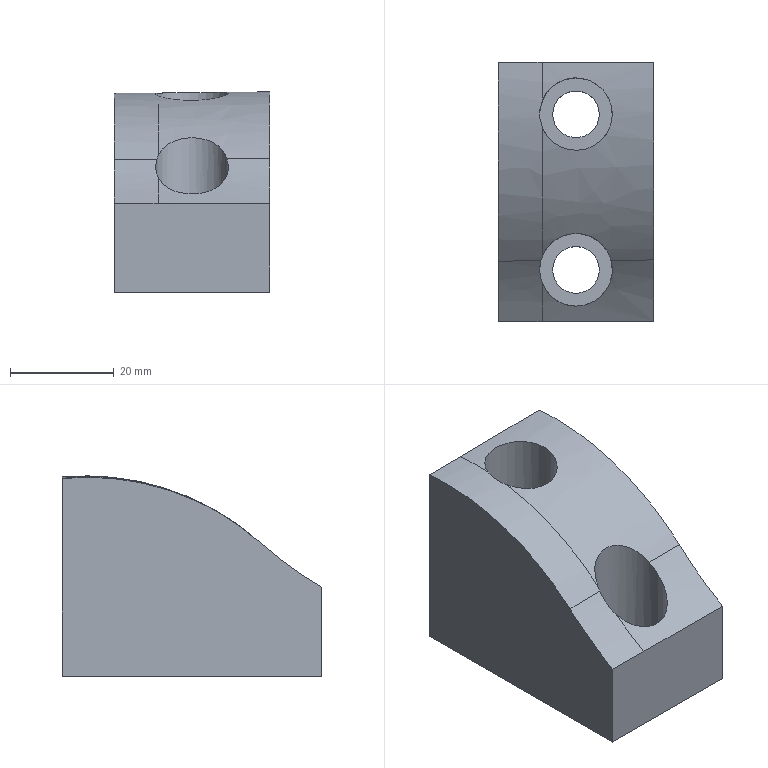Part | NX | features solid 2 | 1 solid | 15 faces | box 30 x 50 x 38.612 mm | volume 39721 mm3 | plane 7 | cylinder 4 | spline 4 | commonest cylinder face diameters 9 x2 14 x2
STEP:
#1=CARTESIAN_POINT('',(470.,654.163,-43.399));
#2=VERTEX_POINT('',#1);
#3=CARTESIAN_POINT('',(470.,642.5,-51.831));
#4=VERTEX_POINT('',#3);
#5=CARTESIAN_POINT('',(470.,654.163,-43.399));
#6=CARTESIAN_POINT('',(470.,650.566,-46.612));
#7=CARTESIAN_POINT('',(470.,646.678,-49.423));
#8=CARTESIAN_POINT('',(470.,642.5,-51.831));
#9=B_SPLINE_CURVE_WITH_KNOTS('',3,(#5,#6,#7,#8),.UNSPECIFIED.,.F.,.F.,(4,4),(0.,0.01439),.UNSPECIFIED.);
#10=EDGE_CURVE('',#2,#4,#9,.T.);
#11=ORIENTED_EDGE('',*,*,#10,.F.);
#12=CARTESIAN_POINT('',(470.,692.5,-30.941));
#13=VERTEX_POINT('',#12);
#14=CARTESIAN_POINT('',(470.,654.163,-43.399));
#15=CARTESIAN_POINT('',(470.,656.729,-41.108));
#16=CARTESIAN_POINT('',(470.,662.388,-37.023));
#17=CARTESIAN_POINT('',(470.,671.861,-32.81));
#18=CARTESIAN_POINT('',(470.,682.125,-30.614));
#19=CARTESIAN_POINT('',(470.,689.029,-30.591));
#20=CARTESIAN_POINT('',(470.,692.5,-30.941));
#21=B_SPLINE_CURVE_WITH_KNOTS('',3,(#14,#15,#16,#17,#18,#19,#20),.UNSPECIFIED.,.F.,.F.,(4,1,1,1,4),(0.007147,0.01746,0.02778,0.0381,0.04842),.UNSPECIFIED.);
#22=EDGE_CURVE('',#2,#13,#21,.T.);
#23=ORIENTED_EDGE('',*,*,#22,.T.);
#24=CARTESIAN_POINT('',(470.,692.5,-69.));
#25=VERTEX_POINT('',#24);
#26=CARTESIAN_POINT('',(470.,692.5,26.));
#27=DIRECTION('',(0.,0.,-1.));
#28=VECTOR('',#27,1000.);
#29=LINE('',#26,#28);
#30=EDGE_CURVE('',#13,#25,#29,.T.);
#31=ORIENTED_EDGE('',*,*,#30,.T.);
#32=CARTESIAN_POINT('',(470.,642.5,-69.));
#33=VERTEX_POINT('',#32);
#34=CARTESIAN_POINT('',(470.,692.5,-69.));
#35=DIRECTION('',(0.,-1.,0.));
#36=VECTOR('',#35,1000.);
#37=LINE('',#34,#36);
#38=EDGE_CURVE('',#25,#33,#37,.T.);
#39=ORIENTED_EDGE('',*,*,#38,.T.);
#40=CARTESIAN_POINT('',(470.,642.5,26.));
#41=DIRECTION('',(0.,0.,-1.));
#42=VECTOR('',#41,1000.);
#43=LINE('',#40,#42);
#44=EDGE_CURVE('',#4,#33,#43,.T.);
#45=ORIENTED_EDGE('',*,*,#44,.F.);
#46=EDGE_LOOP('',(#11,#23,#31,#39,#45));
#47=FACE_BOUND('',#46,.T.);
#48=CARTESIAN_POINT('',(470.,692.5,26.));
#49=DIRECTION('',(1.,0.,0.));
#50=DIRECTION('',(0.,0.,-1.));
#51=AXIS2_PLACEMENT_3D('',#48,#49,#50);
#52=PLANE('',#51);
#53=ADVANCED_FACE('',(#47),#52,.F.);
#54=CARTESIAN_POINT('',(500.,692.5,-30.601));
#55=VERTEX_POINT('',#54);
#56=CARTESIAN_POINT('',(500.,692.5,-69.));
#57=VERTEX_POINT('',#56);
#58=CARTESIAN_POINT('',(500.,692.5,26.));
#59=DIRECTION('',(0.,0.,-1.));
#60=VECTOR('',#59,1000.);
#61=LINE('',#58,#60);
#62=EDGE_CURVE('',#55,#57,#61,.T.);
#63=ORIENTED_EDGE('',*,*,#62,.F.);
#64=CARTESIAN_POINT('',(500.,654.387,-43.29));
#65=VERTEX_POINT('',#64);
#66=CARTESIAN_POINT('',(500.,692.5,-30.601));
#67=CARTESIAN_POINT('',(500.,689.038,-30.282));
#68=CARTESIAN_POINT('',(500.,682.189,-30.36));
#69=CARTESIAN_POINT('',(500.,671.967,-32.624));
#70=CARTESIAN_POINT('',(500.,662.587,-36.865));
#71=CARTESIAN_POINT('',(500.,656.939,-40.985));
#72=CARTESIAN_POINT('',(500.,654.387,-43.291));
#73=B_SPLINE_CURVE_WITH_KNOTS('',3,(#66,#67,#68,#69,#70,#71,#72),.UNSPECIFIED.,.F.,.F.,(4,1,1,1,4),(0.,0.01028,0.02056,0.03084,0.04112),.UNSPECIFIED.);
#74=EDGE_CURVE('',#55,#65,#73,.T.);
#75=ORIENTED_EDGE('',*,*,#74,.T.);
#76=CARTESIAN_POINT('',(500.,642.5,-51.947));
#77=VERTEX_POINT('',#76);
#78=CARTESIAN_POINT('',(500.,642.5,-51.947));
#79=CARTESIAN_POINT('',(500.,646.767,-49.48));
#80=CARTESIAN_POINT('',(500.,650.73,-46.594));
#81=CARTESIAN_POINT('',(500.,654.387,-43.29));
#82=B_SPLINE_CURVE_WITH_KNOTS('',3,(#78,#79,#80,#81),.UNSPECIFIED.,.F.,.F.,(4,4),(0.,0.01471),.UNSPECIFIED.);
#83=EDGE_CURVE('',#77,#65,#82,.T.);
#84=ORIENTED_EDGE('',*,*,#83,.F.);
#85=CARTESIAN_POINT('',(500.,642.5,-69.));
#86=VERTEX_POINT('',#85);
#87=CARTESIAN_POINT('',(500.,642.5,26.));
#88=DIRECTION('',(0.,0.,-1.));
#89=VECTOR('',#88,1000.);
#90=LINE('',#87,#89);
#91=EDGE_CURVE('',#77,#86,#90,.T.);
#92=ORIENTED_EDGE('',*,*,#91,.T.);
#93=CARTESIAN_POINT('',(500.,692.5,-69.));
#94=DIRECTION('',(0.,1.,0.));
#95=VECTOR('',#94,1000.);
#96=LINE('',#93,#95);
#97=EDGE_CURVE('',#57,#86,#96,.F.);
#98=ORIENTED_EDGE('',*,*,#97,.F.);
#99=EDGE_LOOP('',(#63,#75,#84,#92,#98));
#100=FACE_BOUND('',#99,.T.);
#101=CARTESIAN_POINT('',(500.,692.5,26.));
#102=DIRECTION('',(1.,0.,0.));
#103=DIRECTION('',(0.,0.,-1.));
#104=AXIS2_PLACEMENT_3D('',#101,#102,#103);
#105=PLANE('',#104);
#106=ADVANCED_FACE('',(#100),#105,.T.);
#107=CARTESIAN_POINT('',(478.461,692.5,-30.845));
#108=VERTEX_POINT('',#107);
#109=CARTESIAN_POINT('',(470.,692.5,-30.941));
#110=CARTESIAN_POINT('',(472.82,692.5,-30.909));
#111=CARTESIAN_POINT('',(475.641,692.5,-30.877));
#112=CARTESIAN_POINT('',(478.461,692.5,-30.845));
#113=B_SPLINE_CURVE_WITH_KNOTS('',3,(#109,#110,#111,#112),.UNSPECIFIED.,.F.,.F.,(4,4),(0.,0.008461),.UNSPECIFIED.);
#114=EDGE_CURVE('',#13,#108,#113,.T.);
#115=ORIENTED_EDGE('',*,*,#114,.T.);
#116=CARTESIAN_POINT('',(478.461,692.5,-30.845));
#117=CARTESIAN_POINT('',(485.641,692.5,-30.764));
#118=CARTESIAN_POINT('',(492.82,692.5,-30.683));
#119=CARTESIAN_POINT('',(500.,692.5,-30.601));
#120=B_SPLINE_CURVE_WITH_KNOTS('',3,(#116,#117,#118,#119),.UNSPECIFIED.,.F.,.F.,(4,4),(0.001781,0.02332),.UNSPECIFIED.);
#121=EDGE_CURVE('',#108,#55,#120,.T.);
#122=ORIENTED_EDGE('',*,*,#121,.T.);
#123=ORIENTED_EDGE('',*,*,#62,.T.);
#124=CARTESIAN_POINT('',(470.,692.5,-69.));
#125=DIRECTION('',(-1.,0.,0.));
#126=VECTOR('',#125,1000.);
#127=LINE('',#124,#126);
#128=EDGE_CURVE('',#25,#57,#127,.F.);
#129=ORIENTED_EDGE('',*,*,#128,.F.);
#130=ORIENTED_EDGE('',*,*,#30,.F.);
#131=EDGE_LOOP('',(#115,#122,#123,#129,#130));
#132=FACE_BOUND('',#131,.T.);
#133=CARTESIAN_POINT('',(470.,692.5,26.));
#134=DIRECTION('',(0.,1.,0.));
#135=DIRECTION('',(0.,0.,-1.));
#136=AXIS2_PLACEMENT_3D('',#133,#134,#135);
#137=PLANE('',#136);
#138=ADVANCED_FACE('',(#132),#137,.T.);
#139=CARTESIAN_POINT('',(478.,682.5,-59.));
#140=VERTEX_POINT('',#139);
#141=CARTESIAN_POINT('',(485.,682.5,-59.));
#142=DIRECTION('',(0.,0.,-1.));
#143=DIRECTION('',(-1.,0.,0.));
#144=AXIS2_PLACEMENT_3D('',#141,#142,#143);
#145=CIRCLE('',#144,7.);
#146=EDGE_CURVE('',#140,#140,#145,.T.);
#147=ORIENTED_EDGE('',*,*,#146,.T.);
#148=EDGE_LOOP('',(#147));
#149=FACE_BOUND('',#148,.T.);
#150=CARTESIAN_POINT('',(478.461,684.998,-30.673));
#151=VERTEX_POINT('',#150);
#152=CARTESIAN_POINT('',(478.461,680.002,-31.186));
#153=VERTEX_POINT('',#152);
#154=CARTESIAN_POINT('',(478.461,684.998,-30.673));
#155=CARTESIAN_POINT('',(479.04,686.514,-30.589));
#156=CARTESIAN_POINT('',(481.299,689.126,-30.582));
#157=CARTESIAN_POINT('',(486.414,689.957,-30.579));
#158=CARTESIAN_POINT('',(490.872,687.312,-30.43));
#159=CARTESIAN_POINT('',(492.581,682.42,-30.663));
#160=CARTESIAN_POINT('',(490.801,677.632,-31.471));
#161=CARTESIAN_POINT('',(486.374,675.036,-32.165));
#162=CARTESIAN_POINT('',(481.246,675.906,-31.954));
#163=CARTESIAN_POINT('',(479.033,678.504,-31.412));
#164=CARTESIAN_POINT('',(478.461,680.002,-31.186));
#165=B_SPLINE_CURVE_WITH_KNOTS('',3,(#154,#155,#156,#157,#158,#159,#160,#161,#162,#163,#164),.UNSPECIFIED.,.F.,.F.,(4,1,1,1,1,1,1,1,4),(0.01357,0.01842,0.02328,0.02813,0.03298,0.03784,0.04269,0.04755,0.0524),.UNSPECIFIED.);
#166=EDGE_CURVE('',#151,#153,#165,.T.);
#167=ORIENTED_EDGE('',*,*,#166,.F.);
#168=CARTESIAN_POINT('',(478.461,680.002,-31.186));
#169=CARTESIAN_POINT('',(477.855,681.588,-30.947));
#170=CARTESIAN_POINT('',(477.852,683.405,-30.762));
#171=CARTESIAN_POINT('',(478.461,684.998,-30.673));
#172=B_SPLINE_CURVE_WITH_KNOTS('',3,(#168,#169,#170,#171),.UNSPECIFIED.,.F.,.F.,(4,4),(0.0028,0.007913),.UNSPECIFIED.);
#173=EDGE_CURVE('',#153,#151,#172,.T.);
#174=ORIENTED_EDGE('',*,*,#173,.F.);
#175=EDGE_LOOP('',(#167,#174));
#176=FACE_BOUND('',#175,.T.);
#177=CARTESIAN_POINT('',(485.,682.5,26.));
#178=DIRECTION('',(0.,0.,-1.));
#179=DIRECTION('',(0.,-1.,0.));
#180=AXIS2_PLACEMENT_3D('',#177,#178,#179);
#181=CYLINDRICAL_SURFACE('',#180,7.);
#182=ADVANCED_FACE('',(#149,#176),#181,.F.);
#183=CARTESIAN_POINT('',(478.,652.5,-59.));
#184=VERTEX_POINT('',#183);
#185=CARTESIAN_POINT('',(485.,652.5,-59.));
#186=DIRECTION('',(0.,0.,-1.));
#187=DIRECTION('',(-1.,0.,0.));
#188=AXIS2_PLACEMENT_3D('',#185,#186,#187);
#189=CIRCLE('',#188,7.);
#190=EDGE_CURVE('',#184,#184,#189,.T.);
#191=ORIENTED_EDGE('',*,*,#190,.T.);
#192=EDGE_LOOP('',(#191));
#193=FACE_BOUND('',#192,.T.);
#194=CARTESIAN_POINT('',(478.461,654.998,-42.695));
#195=VERTEX_POINT('',#194);
#196=CARTESIAN_POINT('',(491.756,654.33,-43.319));
#197=VERTEX_POINT('',#196);
#198=CARTESIAN_POINT('',(478.461,654.998,-42.695));
#199=CARTESIAN_POINT('',(478.914,656.184,-41.676));
#200=CARTESIAN_POINT('',(480.555,658.558,-39.864));
#201=CARTESIAN_POINT('',(484.662,659.839,-39.021));
#202=CARTESIAN_POINT('',(487.869,659.033,-39.565));
#203=CARTESIAN_POINT('',(490.441,657.323,-40.794));
#204=CARTESIAN_POINT('',(491.434,655.52,-42.247));
#205=CARTESIAN_POINT('',(491.756,654.33,-43.32));
#206=B_SPLINE_CURVE_WITH_KNOTS('',3,(#198,#199,#200,#201,#202,#203,#204,#205),.UNSPECIFIED.,.F.,.F.,(4,1,1,1,1,4),(0.008202,0.01303,0.01785,0.02027,0.02268,0.02751),.UNSPECIFIED.);
#207=EDGE_CURVE('',#195,#197,#206,.T.);
#208=ORIENTED_EDGE('',*,*,#207,.F.);
#209=CARTESIAN_POINT('',(478.217,654.229,-43.369));
#210=VERTEX_POINT('',#209);
#211=CARTESIAN_POINT('',(478.217,654.229,-43.369));
#212=CARTESIAN_POINT('',(478.282,654.485,-43.14));
#213=CARTESIAN_POINT('',(478.363,654.742,-42.915));
#214=CARTESIAN_POINT('',(478.461,654.998,-42.695));
#215=B_SPLINE_CURVE_WITH_KNOTS('',3,(#211,#212,#213,#214),.UNSPECIFIED.,.F.,.F.,(4,4),(0.007158,0.008202),.UNSPECIFIED.);
#216=EDGE_CURVE('',#210,#195,#215,.T.);
#217=ORIENTED_EDGE('',*,*,#216,.F.);
#218=CARTESIAN_POINT('',(478.461,650.002,-46.868));
#219=VERTEX_POINT('',#218);
#220=CARTESIAN_POINT('',(478.217,654.229,-43.369));
#221=CARTESIAN_POINT('',(477.869,652.865,-44.589));
#222=CARTESIAN_POINT('',(477.926,651.402,-45.797));
#223=CARTESIAN_POINT('',(478.461,650.002,-46.868));
#224=B_SPLINE_CURVE_WITH_KNOTS('',3,(#220,#221,#222,#223),.UNSPECIFIED.,.F.,.F.,(4,4),(0.,0.005529),.UNSPECIFIED.);
#225=EDGE_CURVE('',#210,#219,#224,.T.);
#226=ORIENTED_EDGE('',*,*,#225,.T.);
#227=CARTESIAN_POINT('',(478.461,650.002,-46.868));
#228=CARTESIAN_POINT('',(478.749,649.247,-47.445));
#229=CARTESIAN_POINT('',(479.617,647.765,-48.529));
#230=CARTESIAN_POINT('',(481.846,646.024,-49.71));
#231=CARTESIAN_POINT('',(484.817,645.279,-50.197));
#232=CARTESIAN_POINT('',(487.836,645.873,-49.83));
#233=CARTESIAN_POINT('',(490.185,647.54,-48.723));
#234=CARTESIAN_POINT('',(492.054,650.473,-46.609));
#235=CARTESIAN_POINT('',(492.154,652.865,-44.64));
#236=CARTESIAN_POINT('',(491.756,654.331,-43.319));
#237=B_SPLINE_CURVE_WITH_KNOTS('',3,(#227,#228,#229,#230,#231,#232,#233,#234,#235,#236),.UNSPECIFIED.,.F.,.F.,(4,1,1,1,1,1,1,4),(0.005529,0.008511,0.01149,0.01447,0.01746,0.02044,0.02342,0.02938),.UNSPECIFIED.);
#238=EDGE_CURVE('',#219,#197,#237,.T.);
#239=ORIENTED_EDGE('',*,*,#238,.T.);
#240=EDGE_LOOP('',(#208,#217,#226,#239));
#241=FACE_BOUND('',#240,.T.);
#242=CARTESIAN_POINT('',(485.,652.5,26.));
#243=DIRECTION('',(0.,0.,-1.));
#244=DIRECTION('',(0.,-1.,0.));
#245=AXIS2_PLACEMENT_3D('',#242,#243,#244);
#246=CYLINDRICAL_SURFACE('',#245,7.);
#247=ADVANCED_FACE('',(#193,#241),#246,.F.);
#248=CARTESIAN_POINT('',(489.5,652.5,-69.));
#249=VERTEX_POINT('',#248);
#250=CARTESIAN_POINT('',(485.,652.5,-69.));
#251=DIRECTION('',(0.,0.,1.));
#252=DIRECTION('',(1.,0.,0.));
#253=AXIS2_PLACEMENT_3D('',#250,#251,#252);
#254=CIRCLE('',#253,4.5);
#255=EDGE_CURVE('',#249,#249,#254,.F.);
#256=ORIENTED_EDGE('',*,*,#255,.F.);
#257=EDGE_LOOP('',(#256));
#258=FACE_BOUND('',#257,.T.);
#259=CARTESIAN_POINT('',(489.5,682.5,-69.));
#260=VERTEX_POINT('',#259);
#261=CARTESIAN_POINT('',(485.,682.5,-69.));
#262=DIRECTION('',(0.,0.,1.));
#263=DIRECTION('',(1.,0.,0.));
#264=AXIS2_PLACEMENT_3D('',#261,#262,#263);
#265=CIRCLE('',#264,4.5);
#266=EDGE_CURVE('',#260,#260,#265,.F.);
#267=ORIENTED_EDGE('',*,*,#266,.F.);
#268=EDGE_LOOP('',(#267));
#269=FACE_BOUND('',#268,.T.);
#270=ORIENTED_EDGE('',*,*,#38,.F.);
#271=ORIENTED_EDGE('',*,*,#128,.T.);
#272=ORIENTED_EDGE('',*,*,#97,.T.);
#273=CARTESIAN_POINT('',(470.,642.5,-69.));
#274=DIRECTION('',(-1.,0.,0.));
#275=VECTOR('',#274,1000.);
#276=LINE('',#273,#275);
#277=EDGE_CURVE('',#33,#86,#276,.F.);
#278=ORIENTED_EDGE('',*,*,#277,.F.);
#279=EDGE_LOOP('',(#270,#271,#272,#278));
#280=FACE_BOUND('',#279,.T.);
#281=CARTESIAN_POINT('',(470.,692.5,-69.));
#282=DIRECTION('',(0.,0.,1.));
#283=DIRECTION('',(1.,0.,0.));
#284=AXIS2_PLACEMENT_3D('',#281,#282,#283);
#285=PLANE('',#284);
#286=ADVANCED_FACE('',(#258,#269,#280),#285,.F.);
#287=ORIENTED_EDGE('',*,*,#91,.F.);
#288=CARTESIAN_POINT('',(478.461,642.5,-51.865));
#289=VERTEX_POINT('',#288);
#290=CARTESIAN_POINT('',(500.,642.5,-51.947));
#291=CARTESIAN_POINT('',(492.82,642.5,-51.92));
#292=CARTESIAN_POINT('',(485.641,642.5,-51.893));
#293=CARTESIAN_POINT('',(478.461,642.5,-51.865));
#294=B_SPLINE_CURVE_WITH_KNOTS('',3,(#290,#291,#292,#293),.UNSPECIFIED.,.F.,.F.,(4,4),(0.,0.02154),.UNSPECIFIED.);
#295=EDGE_CURVE('',#77,#289,#294,.T.);
#296=ORIENTED_EDGE('',*,*,#295,.T.);
#297=CARTESIAN_POINT('',(478.461,642.5,-51.865));
#298=CARTESIAN_POINT('',(475.641,642.5,-51.854));
#299=CARTESIAN_POINT('',(472.82,642.5,-51.843));
#300=CARTESIAN_POINT('',(470.,642.5,-51.831));
#301=B_SPLINE_CURVE_WITH_KNOTS('',3,(#297,#298,#299,#300),.UNSPECIFIED.,.F.,.F.,(4,4),(0.001317,0.009778),.UNSPECIFIED.);
#302=EDGE_CURVE('',#289,#4,#301,.T.);
#303=ORIENTED_EDGE('',*,*,#302,.T.);
#304=ORIENTED_EDGE('',*,*,#44,.T.);
#305=ORIENTED_EDGE('',*,*,#277,.T.);
#306=EDGE_LOOP('',(#287,#296,#303,#304,#305));
#307=FACE_BOUND('',#306,.T.);
#308=CARTESIAN_POINT('',(470.,642.5,26.));
#309=DIRECTION('',(0.,1.,0.));
#310=DIRECTION('',(0.,0.,-1.));
#311=AXIS2_PLACEMENT_3D('',#308,#309,#310);
#312=PLANE('',#311);
#313=ADVANCED_FACE('',(#307),#312,.F.);
#314=ORIENTED_EDGE('',*,*,#266,.T.);
#315=EDGE_LOOP('',(#314));
#316=FACE_BOUND('',#315,.T.);
#317=CARTESIAN_POINT('',(480.5,682.5,-59.));
#318=VERTEX_POINT('',#317);
#319=CARTESIAN_POINT('',(485.,682.5,-59.));
#320=DIRECTION('',(0.,0.,-1.));
#321=DIRECTION('',(-1.,0.,0.));
#322=AXIS2_PLACEMENT_3D('',#319,#320,#321);
#323=CIRCLE('',#322,4.5);
#324=EDGE_CURVE('',#318,#318,#323,.T.);
#325=ORIENTED_EDGE('',*,*,#324,.F.);
#326=EDGE_LOOP('',(#325));
#327=FACE_BOUND('',#326,.T.);
#328=CARTESIAN_POINT('',(485.,682.5,-124.));
#329=DIRECTION('',(0.,0.,-1.));
#330=DIRECTION('',(0.,-1.,0.));
#331=AXIS2_PLACEMENT_3D('',#328,#329,#330);
#332=CYLINDRICAL_SURFACE('',#331,4.5);
#333=ADVANCED_FACE('',(#316,#327),#332,.F.);
#334=ORIENTED_EDGE('',*,*,#324,.T.);
#335=EDGE_LOOP('',(#334));
#336=FACE_BOUND('',#335,.T.);
#337=ORIENTED_EDGE('',*,*,#146,.F.);
#338=EDGE_LOOP('',(#337));
#339=FACE_BOUND('',#338,.T.);
#340=CARTESIAN_POINT('',(485.,682.5,-59.));
#341=DIRECTION('',(0.,0.,-1.));
#342=DIRECTION('',(0.,-1.,0.));
#343=AXIS2_PLACEMENT_3D('',#340,#341,#342);
#344=PLANE('',#343);
#345=ADVANCED_FACE('',(#336,#339),#344,.F.);
#346=ORIENTED_EDGE('',*,*,#255,.T.);
#347=EDGE_LOOP('',(#346));
#348=FACE_BOUND('',#347,.T.);
#349=CARTESIAN_POINT('',(480.5,652.5,-59.));
#350=VERTEX_POINT('',#349);
#351=CARTESIAN_POINT('',(485.,652.5,-59.));
#352=DIRECTION('',(0.,0.,-1.));
#353=DIRECTION('',(-1.,0.,0.));
#354=AXIS2_PLACEMENT_3D('',#351,#352,#353);
#355=CIRCLE('',#354,4.5);
#356=EDGE_CURVE('',#350,#350,#355,.T.);
#357=ORIENTED_EDGE('',*,*,#356,.F.);
#358=EDGE_LOOP('',(#357));
#359=FACE_BOUND('',#358,.T.);
#360=CARTESIAN_POINT('',(485.,652.5,-124.));
#361=DIRECTION('',(0.,0.,-1.));
#362=DIRECTION('',(0.,-1.,0.));
#363=AXIS2_PLACEMENT_3D('',#360,#361,#362);
#364=CYLINDRICAL_SURFACE('',#363,4.5);
#365=ADVANCED_FACE('',(#348,#359),#364,.F.);
#366=ORIENTED_EDGE('',*,*,#356,.T.);
#367=EDGE_LOOP('',(#366));
#368=FACE_BOUND('',#367,.T.);
#369=ORIENTED_EDGE('',*,*,#190,.F.);
#370=EDGE_LOOP('',(#369));
#371=FACE_BOUND('',#370,.T.);
#372=CARTESIAN_POINT('',(485.,652.5,-59.));
#373=DIRECTION('',(0.,0.,-1.));
#374=DIRECTION('',(0.,-1.,0.));
#375=AXIS2_PLACEMENT_3D('',#372,#373,#374);
#376=PLANE('',#375);
#377=ADVANCED_FACE('',(#368,#371),#376,.F.);
#378=ORIENTED_EDGE('',*,*,#74,.F.);
#379=ORIENTED_EDGE('',*,*,#121,.F.);
#380=CARTESIAN_POINT('',(478.461,692.5,-30.845));
#381=CARTESIAN_POINT('',(478.461,690.002,-30.6));
#382=CARTESIAN_POINT('',(478.461,687.501,-30.542));
#383=CARTESIAN_POINT('',(478.461,684.998,-30.673));
#384=B_SPLINE_CURVE_WITH_KNOTS('',3,(#380,#381,#382,#383),.UNSPECIFIED.,.F.,.F.,(4,4),(0.004213,0.01172),.UNSPECIFIED.);
#385=EDGE_CURVE('',#108,#151,#384,.T.);
#386=ORIENTED_EDGE('',*,*,#385,.T.);
#387=ORIENTED_EDGE('',*,*,#166,.T.);
#388=CARTESIAN_POINT('',(478.461,680.002,-31.186));
#389=CARTESIAN_POINT('',(478.461,675.364,-31.899));
#390=CARTESIAN_POINT('',(478.461,668.715,-33.897));
#391=CARTESIAN_POINT('',(478.461,660.457,-38.419));
#392=CARTESIAN_POINT('',(478.461,656.755,-41.184));
#393=CARTESIAN_POINT('',(478.461,654.998,-42.695));
#394=B_SPLINE_CURVE_WITH_KNOTS('',3,(#388,#389,#390,#391,#392,#393),.UNSPECIFIED.,.F.,.F.,(4,1,1,4),(0.01671,0.03059,0.03753,0.04447),.UNSPECIFIED.);
#395=EDGE_CURVE('',#153,#195,#394,.T.);
#396=ORIENTED_EDGE('',*,*,#395,.T.);
#397=ORIENTED_EDGE('',*,*,#207,.T.);
#398=CARTESIAN_POINT('',(500.,654.387,-43.291));
#399=CARTESIAN_POINT('',(497.212,654.368,-43.3));
#400=CARTESIAN_POINT('',(494.464,654.349,-43.31));
#401=CARTESIAN_POINT('',(491.756,654.33,-43.32));
#402=B_SPLINE_CURVE_WITH_KNOTS('',3,(#398,#399,#400,#401),.UNSPECIFIED.,.F.,.F.,(4,4),(0.8538,0.9084),.UNSPECIFIED.);
#403=EDGE_CURVE('',#65,#197,#402,.T.);
#404=ORIENTED_EDGE('',*,*,#403,.F.);
#405=EDGE_LOOP('',(#378,#379,#386,#387,#396,#397,#404));
#406=FACE_BOUND('',#405,.T.);
#407=CARTESIAN_POINT('',(500.126,693.052,-30.654));
#408=CARTESIAN_POINT('',(500.412,670.763,-28.348));
#409=CARTESIAN_POINT('',(500.792,654.213,-43.451));
#410=CARTESIAN_POINT('',(492.636,692.95,-30.729));
#411=CARTESIAN_POINT('',(492.928,670.661,-28.422));
#412=CARTESIAN_POINT('',(493.313,654.109,-43.526));
#413=CARTESIAN_POINT('',(485.145,692.845,-30.804));
#414=CARTESIAN_POINT('',(485.444,670.555,-28.496));
#415=CARTESIAN_POINT('',(485.833,654.002,-43.6));
#416=CARTESIAN_POINT('',(477.655,692.737,-30.878));
#417=CARTESIAN_POINT('',(477.961,670.446,-28.569));
#418=CARTESIAN_POINT('',(478.354,653.892,-43.674));
#419=(BOUNDED_SURFACE()B_SPLINE_SURFACE(3,2,((#407,#408,#409),(#410,#411,#412),(#413,#414,#415),(#416,#417,#418)),.UNSPECIFIED.,.F.,.F.,.F.)B_SPLINE_SURFACE_WITH_KNOTS((4,4),(3,3),(0.3604,0.3829),(0.07856,0.8701),.PIECEWISE_BEZIER_KNOTS.)GEOMETRIC_REPRESENTATION_ITEM()RATIONAL_B_SPLINE_SURFACE(((0.9803,0.8895,0.9692),(0.9803,0.8895,0.9692),(0.9803,0.8895,0.9692),(0.9803,0.8895,0.9692)))REPRESENTATION_ITEM('')SURFACE());
#420=ADVANCED_FACE('',(#406),#419,.T.);
#421=ORIENTED_EDGE('',*,*,#22,.F.);
#422=CARTESIAN_POINT('',(478.217,654.229,-43.369));
#423=CARTESIAN_POINT('',(475.468,654.208,-43.379));
#424=CARTESIAN_POINT('',(472.729,654.185,-43.389));
#425=CARTESIAN_POINT('',(470.,654.163,-43.399));
#426=B_SPLINE_CURVE_WITH_KNOTS('',3,(#422,#423,#424,#425),.UNSPECIFIED.,.F.,.F.,(4,4),(0.001111,0.03868),.UNSPECIFIED.);
#427=EDGE_CURVE('',#210,#2,#426,.T.);
#428=ORIENTED_EDGE('',*,*,#427,.F.);
#429=ORIENTED_EDGE('',*,*,#216,.T.);
#430=ORIENTED_EDGE('',*,*,#395,.F.);
#431=ORIENTED_EDGE('',*,*,#173,.T.);
#432=ORIENTED_EDGE('',*,*,#385,.F.);
#433=ORIENTED_EDGE('',*,*,#114,.F.);
#434=EDGE_LOOP('',(#421,#428,#429,#430,#431,#432,#433));
#435=FACE_BOUND('',#434,.T.);
#436=CARTESIAN_POINT('',(478.511,692.872,-30.883));
#437=CARTESIAN_POINT('',(478.815,670.637,-28.524));
#438=CARTESIAN_POINT('',(479.207,654.059,-43.526));
#439=CARTESIAN_POINT('',(475.421,692.828,-30.913));
#440=CARTESIAN_POINT('',(475.728,670.592,-28.554));
#441=CARTESIAN_POINT('',(476.122,654.013,-43.556));
#442=CARTESIAN_POINT('',(472.331,692.783,-30.944));
#443=CARTESIAN_POINT('',(472.641,670.547,-28.584));
#444=CARTESIAN_POINT('',(473.036,653.967,-43.586));
#445=CARTESIAN_POINT('',(469.241,692.737,-30.974));
#446=CARTESIAN_POINT('',(469.553,670.5,-28.614));
#447=CARTESIAN_POINT('',(469.951,653.921,-43.617));
#448=(BOUNDED_SURFACE()B_SPLINE_SURFACE(3,2,((#436,#437,#438),(#439,#440,#441),(#442,#443,#444),(#445,#446,#447)),.UNSPECIFIED.,.F.,.F.,.F.)B_SPLINE_SURFACE_WITH_KNOTS((4,4),(3,3),(0.382,0.3913),(0.07616,0.8661),.PIECEWISE_BEZIER_KNOTS.)GEOMETRIC_REPRESENTATION_ITEM()RATIONAL_B_SPLINE_SURFACE(((0.9808,0.8897,0.9684),(0.9808,0.8897,0.9684),(0.9808,0.8897,0.9684),(0.9808,0.8897,0.9684)))REPRESENTATION_ITEM('')SURFACE());
#449=ADVANCED_FACE('',(#435),#448,.T.);
#450=ORIENTED_EDGE('',*,*,#295,.F.);
#451=ORIENTED_EDGE('',*,*,#83,.T.);
#452=ORIENTED_EDGE('',*,*,#403,.T.);
#453=ORIENTED_EDGE('',*,*,#238,.F.);
#454=CARTESIAN_POINT('',(478.461,642.5,-51.865));
#455=CARTESIAN_POINT('',(478.461,645.108,-50.361));
#456=CARTESIAN_POINT('',(478.461,647.615,-48.69));
#457=CARTESIAN_POINT('',(478.461,650.002,-46.868));
#458=B_SPLINE_CURVE_WITH_KNOTS('',3,(#454,#455,#456,#457),.UNSPECIFIED.,.F.,.F.,(4,4),(0.04622,0.05514),.UNSPECIFIED.);
#459=EDGE_CURVE('',#289,#219,#458,.T.);
#460=ORIENTED_EDGE('',*,*,#459,.F.);
#461=EDGE_LOOP('',(#450,#451,#452,#453,#460));
#462=FACE_BOUND('',#461,.T.);
#463=CARTESIAN_POINT('',(500.129,642.425,-51.99));
#464=CARTESIAN_POINT('',(500.173,648.869,-48.276));
#465=CARTESIAN_POINT('',(500.221,654.389,-43.289));
#466=CARTESIAN_POINT('',(492.851,642.386,-51.986));
#467=CARTESIAN_POINT('',(492.89,648.823,-48.285));
#468=CARTESIAN_POINT('',(492.933,654.34,-43.315));
#469=CARTESIAN_POINT('',(485.572,642.342,-51.984));
#470=CARTESIAN_POINT('',(485.606,648.773,-48.295));
#471=CARTESIAN_POINT('',(485.645,654.288,-43.341));
#472=CARTESIAN_POINT('',(478.292,642.294,-51.983));
#473=CARTESIAN_POINT('',(478.322,648.718,-48.306));
#474=CARTESIAN_POINT('',(478.356,654.23,-43.368));
#475=(BOUNDED_SURFACE()B_SPLINE_SURFACE(3,2,((#463,#464,#465),(#466,#467,#468),(#469,#470,#471),(#472,#473,#474)),.UNSPECIFIED.,.F.,.F.,.F.)B_SPLINE_SURFACE_WITH_KNOTS((4,4),(3,3),(0.3549,0.3768),(0.755,1.),.PIECEWISE_BEZIER_KNOTS.)GEOMETRIC_REPRESENTATION_ITEM()RATIONAL_B_SPLINE_SURFACE(((0.9652,0.9769,1.),(0.9653,0.977,1.),(0.9654,0.9771,1.),(0.9655,0.9772,1.)))REPRESENTATION_ITEM('')SURFACE());
#476=ADVANCED_FACE('',(#462),#475,.F.);
#477=ORIENTED_EDGE('',*,*,#427,.T.);
#478=ORIENTED_EDGE('',*,*,#10,.T.);
#479=ORIENTED_EDGE('',*,*,#302,.F.);
#480=ORIENTED_EDGE('',*,*,#459,.T.);
#481=ORIENTED_EDGE('',*,*,#225,.F.);
#482=EDGE_LOOP('',(#477,#478,#479,#480,#481));
#483=FACE_BOUND('',#482,.T.);
#484=CARTESIAN_POINT('',(478.512,642.425,-51.908));
#485=CARTESIAN_POINT('',(478.542,648.776,-48.256));
#486=CARTESIAN_POINT('',(478.576,654.232,-43.367));
#487=CARTESIAN_POINT('',(475.64,642.406,-51.908));
#488=CARTESIAN_POINT('',(475.668,648.754,-48.26));
#489=CARTESIAN_POINT('',(475.7,654.21,-43.378));
#490=CARTESIAN_POINT('',(472.768,642.386,-51.908));
#491=CARTESIAN_POINT('',(472.794,648.732,-48.265));
#492=CARTESIAN_POINT('',(472.825,654.186,-43.389));
#493=CARTESIAN_POINT('',(469.896,642.366,-51.908));
#494=CARTESIAN_POINT('',(469.92,648.708,-48.27));
#495=CARTESIAN_POINT('',(469.949,654.162,-43.4));
#496=(BOUNDED_SURFACE()B_SPLINE_SURFACE(3,2,((#484,#485,#486),(#487,#488,#489),(#490,#491,#492),(#493,#494,#495)),.UNSPECIFIED.,.F.,.F.,.F.)B_SPLINE_SURFACE_WITH_KNOTS((4,4),(3,3),(0.3765,0.3852),(0.7574,1.),.PIECEWISE_BEZIER_KNOTS.)GEOMETRIC_REPRESENTATION_ITEM()RATIONAL_B_SPLINE_SURFACE(((0.9657,0.9774,1.),(0.9658,0.9774,1.),(0.9658,0.9774,1.),(0.9659,0.9775,1.)))REPRESENTATION_ITEM('')SURFACE());
#497=ADVANCED_FACE('',(#483),#496,.F.);
#498=CLOSED_SHELL('',(#53,#106,#138,#182,#247,#286,#313,#333,#345,#365,#377,#420,#449,#476,#497));
#499=MANIFOLD_SOLID_BREP('',#498);
#500=(LENGTH_UNIT()NAMED_UNIT(*)SI_UNIT(.MILLI.,.METRE.));
#501=UNCERTAINTY_MEASURE_WITH_UNIT(LENGTH_MEASURE(0.05201),#500,'','');
#502=(NAMED_UNIT(*)PLANE_ANGLE_UNIT()SI_UNIT($,.RADIAN.));
#503=(NAMED_UNIT(*)SI_UNIT($,.STERADIAN.)SOLID_ANGLE_UNIT());
#504=(GEOMETRIC_REPRESENTATION_CONTEXT(3)GLOBAL_UNCERTAINTY_ASSIGNED_CONTEXT((#501))GLOBAL_UNIT_ASSIGNED_CONTEXT((#500,#502,#503))REPRESENTATION_CONTEXT('',''));
#505=ADVANCED_BREP_SHAPE_REPRESENTATION('',(#499),#504);